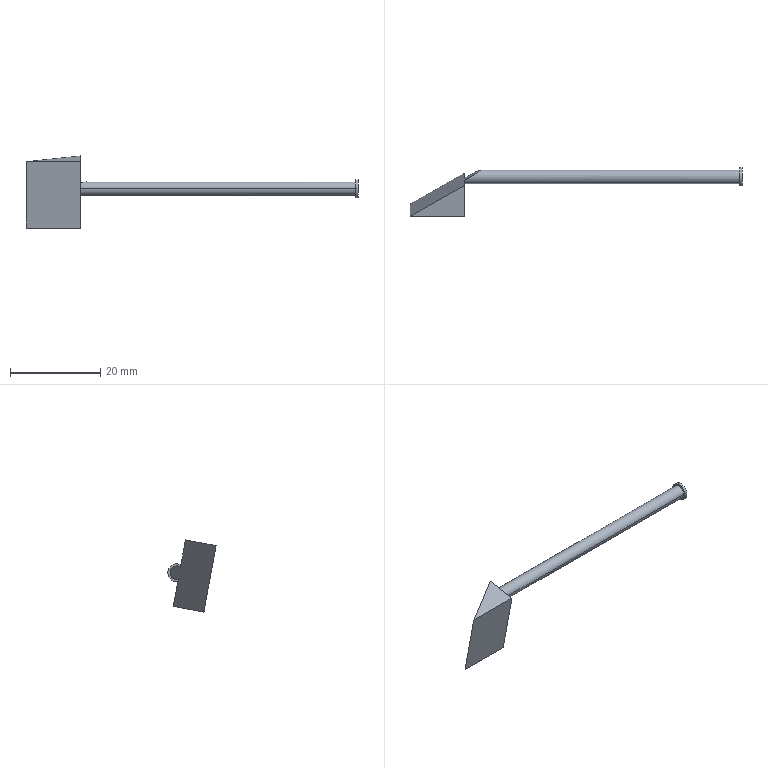Part | SolidWorks | features ICE 4, Cut 1, Helix 1, Revolution 1, Scale 1, SweepCut 1 | 1 solid | 11 faces | box 73.75 x 10.739 x 16.01 mm | volume 1055 mm3 | plane 7 | cylinder 4 | commonest cylinder face diameters 3 x2 4 x2
STEP:
#1=CARTESIAN_POINT('',(42.25,-1.5,0.));
#2=VERTEX_POINT('',#1);
#3=CARTESIAN_POINT('',(42.25,1.5,0.));
#4=VERTEX_POINT('',#3);
#5=CARTESIAN_POINT('',(42.25,0.,0.));
#6=DIRECTION('',(-1.,0.,0.));
#7=DIRECTION('',(0.,-1.,0.));
#8=AXIS2_PLACEMENT_3D('',#5,#6,#7);
#9=CIRCLE('',#8,1.5);
#10=EDGE_CURVE('',#2,#4,#9,.T.);
#11=ORIENTED_EDGE('',*,*,#10,.T.);
#12=CARTESIAN_POINT('',(-15.455,1.5,0.));
#13=VERTEX_POINT('',#12);
#14=CARTESIAN_POINT('',(-11.,1.5,0.));
#15=DIRECTION('',(-1.,0.,0.));
#16=VECTOR('',#15,1000.);
#17=LINE('',#14,#16);
#18=EDGE_CURVE('',#4,#13,#17,.T.);
#19=ORIENTED_EDGE('',*,*,#18,.T.);
#20=CARTESIAN_POINT('',(-19.,-0.8145,1.26));
#21=VERTEX_POINT('',#20);
#22=CARTESIAN_POINT('',(-15.455,1.5,0.));
#23=CARTESIAN_POINT('',(-15.031,1.5,1.347));
#24=CARTESIAN_POINT('',(-16.843,0.3168,1.991));
#25=CARTESIAN_POINT('',(-19.,-0.8145,1.26));
#26=(BOUNDED_CURVE()B_SPLINE_CURVE(3,(#22,#23,#24,#25),.UNSPECIFIED.,.F.,.F.)B_SPLINE_CURVE_WITH_KNOTS((4,4),(2.959,5.103),.UNSPECIFIED.)CURVE()GEOMETRIC_REPRESENTATION_ITEM()RATIONAL_B_SPLINE_CURVE((1.,0.652,0.652,1.))REPRESENTATION_ITEM(''));
#27=EDGE_CURVE('',#13,#21,#26,.T.);
#28=ORIENTED_EDGE('',*,*,#27,.T.);
#29=CARTESIAN_POINT('',(-19.,-1.5,0.));
#30=VERTEX_POINT('',#29);
#31=CARTESIAN_POINT('',(-19.,0.,0.));
#32=DIRECTION('',(-1.,0.,0.));
#33=DIRECTION('',(0.,0.,1.));
#34=AXIS2_PLACEMENT_3D('',#31,#32,#33);
#35=CIRCLE('',#34,1.5);
#36=EDGE_CURVE('',#30,#21,#35,.T.);
#37=ORIENTED_EDGE('',*,*,#36,.F.);
#38=CARTESIAN_POINT('',(-11.,-1.5,0.));
#39=DIRECTION('',(-1.,0.,0.));
#40=VECTOR('',#39,1000.);
#41=LINE('',#38,#40);
#42=EDGE_CURVE('',#2,#30,#41,.T.);
#43=ORIENTED_EDGE('',*,*,#42,.F.);
#44=EDGE_LOOP('',(#11,#19,#28,#37,#43));
#45=FACE_OUTER_BOUND('',#44,.T.);
#46=CARTESIAN_POINT('',(-11.,0.,0.));
#47=DIRECTION('',(-1.,0.,0.));
#48=DIRECTION('',(0.,-1.,0.));
#49=AXIS2_PLACEMENT_3D('',#46,#47,#48);
#50=CYLINDRICAL_SURFACE('',#49,1.5);
#51=ADVANCED_FACE('',(#45),#50,.T.);
#52=CARTESIAN_POINT('',(42.75,-2.,0.));
#53=VERTEX_POINT('',#52);
#54=CARTESIAN_POINT('',(42.75,2.,0.));
#55=VERTEX_POINT('',#54);
#56=CARTESIAN_POINT('',(42.75,0.,0.));
#57=DIRECTION('',(-1.,0.,0.));
#58=DIRECTION('',(0.,-1.,0.));
#59=AXIS2_PLACEMENT_3D('',#56,#57,#58);
#60=CIRCLE('',#59,2.);
#61=EDGE_CURVE('',#53,#55,#60,.T.);
#62=ORIENTED_EDGE('',*,*,#61,.T.);
#63=CARTESIAN_POINT('',(42.25,2.,0.));
#64=VERTEX_POINT('',#63);
#65=CARTESIAN_POINT('',(-11.,2.,0.));
#66=DIRECTION('',(-1.,0.,0.));
#67=VECTOR('',#66,1000.);
#68=LINE('',#65,#67);
#69=EDGE_CURVE('',#55,#64,#68,.T.);
#70=ORIENTED_EDGE('',*,*,#69,.T.);
#71=CARTESIAN_POINT('',(42.25,-2.,0.));
#72=VERTEX_POINT('',#71);
#73=CARTESIAN_POINT('',(42.25,0.,0.));
#74=DIRECTION('',(-1.,0.,0.));
#75=DIRECTION('',(0.,-1.,0.));
#76=AXIS2_PLACEMENT_3D('',#73,#74,#75);
#77=CIRCLE('',#76,2.);
#78=EDGE_CURVE('',#72,#64,#77,.T.);
#79=ORIENTED_EDGE('',*,*,#78,.F.);
#80=CARTESIAN_POINT('',(-11.,-2.,0.));
#81=DIRECTION('',(-1.,0.,0.));
#82=VECTOR('',#81,1000.);
#83=LINE('',#80,#82);
#84=EDGE_CURVE('',#53,#72,#83,.T.);
#85=ORIENTED_EDGE('',*,*,#84,.F.);
#86=EDGE_LOOP('',(#62,#70,#79,#85));
#87=FACE_OUTER_BOUND('',#86,.T.);
#88=CARTESIAN_POINT('',(-11.,0.,0.));
#89=DIRECTION('',(-1.,0.,0.));
#90=DIRECTION('',(0.,-1.,0.));
#91=AXIS2_PLACEMENT_3D('',#88,#89,#90);
#92=CYLINDRICAL_SURFACE('',#91,2.);
#93=ADVANCED_FACE('',(#87),#92,.T.);
#94=ORIENTED_EDGE('',*,*,#10,.F.);
#95=CARTESIAN_POINT('',(42.25,0.,0.));
#96=DIRECTION('',(-1.,0.,0.));
#97=DIRECTION('',(0.,-1.,0.));
#98=AXIS2_PLACEMENT_3D('',#95,#96,#97);
#99=CIRCLE('',#98,1.5);
#100=EDGE_CURVE('',#4,#2,#99,.T.);
#101=ORIENTED_EDGE('',*,*,#100,.F.);
#102=EDGE_LOOP('',(#94,#101));
#103=FACE_BOUND('',#102,.T.);
#104=ORIENTED_EDGE('',*,*,#78,.T.);
#105=CARTESIAN_POINT('',(42.25,0.,0.));
#106=DIRECTION('',(-1.,0.,0.));
#107=DIRECTION('',(0.,-1.,0.));
#108=AXIS2_PLACEMENT_3D('',#105,#106,#107);
#109=CIRCLE('',#108,2.);
#110=EDGE_CURVE('',#64,#72,#109,.T.);
#111=ORIENTED_EDGE('',*,*,#110,.T.);
#112=EDGE_LOOP('',(#104,#111));
#113=FACE_OUTER_BOUND('',#112,.T.);
#114=CARTESIAN_POINT('',(42.25,1.5,0.));
#115=DIRECTION('',(1.,0.,0.));
#116=DIRECTION('',(0.,1.,0.));
#117=AXIS2_PLACEMENT_3D('',#114,#115,#116);
#118=PLANE('',#117);
#119=ADVANCED_FACE('',(#103,#113),#118,.F.);
#120=ORIENTED_EDGE('',*,*,#69,.F.);
#121=CARTESIAN_POINT('',(42.75,0.,0.));
#122=DIRECTION('',(-1.,0.,0.));
#123=DIRECTION('',(0.,-1.,0.));
#124=AXIS2_PLACEMENT_3D('',#121,#122,#123);
#125=CIRCLE('',#124,2.);
#126=EDGE_CURVE('',#55,#53,#125,.T.);
#127=ORIENTED_EDGE('',*,*,#126,.T.);
#128=ORIENTED_EDGE('',*,*,#84,.T.);
#129=ORIENTED_EDGE('',*,*,#110,.F.);
#130=EDGE_LOOP('',(#120,#127,#128,#129));
#131=FACE_OUTER_BOUND('',#130,.T.);
#132=CARTESIAN_POINT('',(-11.,0.,0.));
#133=DIRECTION('',(-1.,0.,0.));
#134=DIRECTION('',(0.,-1.,0.));
#135=AXIS2_PLACEMENT_3D('',#132,#133,#134);
#136=CYLINDRICAL_SURFACE('',#135,2.);
#137=ADVANCED_FACE('',(#131),#136,.T.);
#138=ORIENTED_EDGE('',*,*,#61,.F.);
#139=ORIENTED_EDGE('',*,*,#126,.F.);
#140=EDGE_LOOP('',(#138,#139));
#141=FACE_OUTER_BOUND('',#140,.T.);
#142=CARTESIAN_POINT('',(42.75,2.,0.));
#143=DIRECTION('',(-1.,0.,0.));
#144=DIRECTION('',(0.,-1.,0.));
#145=AXIS2_PLACEMENT_3D('',#142,#143,#144);
#146=PLANE('',#145);
#147=ADVANCED_FACE('',(#141),#146,.F.);
#148=ORIENTED_EDGE('',*,*,#18,.F.);
#149=ORIENTED_EDGE('',*,*,#100,.T.);
#150=ORIENTED_EDGE('',*,*,#42,.T.);
#151=CARTESIAN_POINT('',(-19.,-0.31,-1.468));
#152=VERTEX_POINT('',#151);
#153=CARTESIAN_POINT('',(-19.,0.,0.));
#154=DIRECTION('',(-1.,0.,0.));
#155=DIRECTION('',(0.,0.,1.));
#156=AXIS2_PLACEMENT_3D('',#153,#154,#155);
#157=CIRCLE('',#156,1.5);
#158=EDGE_CURVE('',#152,#30,#157,.T.);
#159=ORIENTED_EDGE('',*,*,#158,.F.);
#160=CARTESIAN_POINT('',(-19.,-0.31,-1.468));
#161=CARTESIAN_POINT('',(-17.349,0.699,-1.681));
#162=CARTESIAN_POINT('',(-15.78,1.5,-1.031));
#163=CARTESIAN_POINT('',(-15.455,1.5,0.));
#164=(BOUNDED_CURVE()B_SPLINE_CURVE(3,(#160,#161,#162,#163),.UNSPECIFIED.,.F.,.F.)B_SPLINE_CURVE_WITH_KNOTS((4,4),(1.18,2.959),.UNSPECIFIED.)CURVE()GEOMETRIC_REPRESENTATION_ITEM()RATIONAL_B_SPLINE_CURVE((1.,0.7532,0.7532,1.))REPRESENTATION_ITEM(''));
#165=EDGE_CURVE('',#152,#13,#164,.T.);
#166=ORIENTED_EDGE('',*,*,#165,.T.);
#167=EDGE_LOOP('',(#148,#149,#150,#159,#166));
#168=FACE_OUTER_BOUND('',#167,.T.);
#169=CARTESIAN_POINT('',(-11.,0.,0.));
#170=DIRECTION('',(-1.,0.,0.));
#171=DIRECTION('',(0.,-1.,0.));
#172=AXIS2_PLACEMENT_3D('',#169,#170,#171);
#173=CYLINDRICAL_SURFACE('',#172,1.5);
#174=ADVANCED_FACE('',(#168),#173,.T.);
#175=CARTESIAN_POINT('',(-19.,-6.011,-8.739));
#176=VERTEX_POINT('',#175);
#177=CARTESIAN_POINT('',(-19.,-8.739,6.011));
#178=VERTEX_POINT('',#177);
#179=CARTESIAN_POINT('',(-19.,-8.739,6.011));
#180=DIRECTION('',(0.,-0.1819,0.9833));
#181=VECTOR('',#180,1000.);
#182=LINE('',#179,#181);
#183=EDGE_CURVE('',#176,#178,#182,.T.);
#184=ORIENTED_EDGE('',*,*,#183,.T.);
#185=CARTESIAN_POINT('',(-31.,-8.739,6.011));
#186=VERTEX_POINT('',#185);
#187=CARTESIAN_POINT('',(-31.,-8.739,6.011));
#188=DIRECTION('',(1.,0.,0.));
#189=VECTOR('',#188,1000.);
#190=LINE('',#187,#189);
#191=EDGE_CURVE('',#186,#178,#190,.T.);
#192=ORIENTED_EDGE('',*,*,#191,.F.);
#193=CARTESIAN_POINT('',(-31.,-6.011,-8.739));
#194=VERTEX_POINT('',#193);
#195=CARTESIAN_POINT('',(-31.,-8.739,6.011));
#196=DIRECTION('',(0.,-0.1819,0.9833));
#197=VECTOR('',#196,1000.);
#198=LINE('',#195,#197);
#199=EDGE_CURVE('',#194,#186,#198,.T.);
#200=ORIENTED_EDGE('',*,*,#199,.F.);
#201=CARTESIAN_POINT('',(-31.,-6.011,-8.739));
#202=DIRECTION('',(1.,0.,0.));
#203=VECTOR('',#202,1000.);
#204=LINE('',#201,#203);
#205=EDGE_CURVE('',#194,#176,#204,.T.);
#206=ORIENTED_EDGE('',*,*,#205,.T.);
#207=EDGE_LOOP('',(#184,#192,#200,#206));
#208=FACE_OUTER_BOUND('',#207,.T.);
#209=CARTESIAN_POINT('',(-31.,-8.739,6.011));
#210=DIRECTION('',(0.,0.9833,0.1819));
#211=DIRECTION('',(0.,-0.1819,0.9833));
#212=AXIS2_PLACEMENT_3D('',#209,#210,#211);
#213=PLANE('',#212);
#214=ADVANCED_FACE('',(#208),#213,.F.);
#215=CARTESIAN_POINT('',(-19.,-1.926,7.271));
#216=VERTEX_POINT('',#215);
#217=CARTESIAN_POINT('',(-19.,6.011,8.739));
#218=DIRECTION('',(0.,0.9833,0.1819));
#219=VECTOR('',#218,1000.);
#220=LINE('',#217,#219);
#221=EDGE_CURVE('',#178,#216,#220,.T.);
#222=ORIENTED_EDGE('',*,*,#221,.T.);
#223=CARTESIAN_POINT('',(-24.505,-5.052,6.693));
#224=DIRECTION('',(-0.866,-0.4917,-0.09094));
#225=VECTOR('',#224,1000.);
#226=LINE('',#223,#225);
#227=EDGE_CURVE('',#216,#186,#226,.T.);
#228=ORIENTED_EDGE('',*,*,#227,.T.);
#229=ORIENTED_EDGE('',*,*,#191,.T.);
#230=EDGE_LOOP('',(#222,#228,#229));
#231=FACE_OUTER_BOUND('',#230,.T.);
#232=CARTESIAN_POINT('',(-31.,6.011,8.739));
#233=DIRECTION('',(0.,0.1819,-0.9833));
#234=DIRECTION('',(0.,0.9833,0.1819));
#235=AXIS2_PLACEMENT_3D('',#232,#233,#234);
#236=PLANE('',#235);
#237=ADVANCED_FACE('',(#231),#236,.F.);
#238=ORIENTED_EDGE('',*,*,#205,.F.);
#239=CARTESIAN_POINT('',(-19.,0.8018,-7.479));
#240=VERTEX_POINT('',#239);
#241=CARTESIAN_POINT('',(-5.019,8.739,-6.011));
#242=DIRECTION('',(-0.866,-0.4917,-0.09094));
#243=VECTOR('',#242,1000.);
#244=LINE('',#241,#243);
#245=EDGE_CURVE('',#240,#194,#244,.T.);
#246=ORIENTED_EDGE('',*,*,#245,.F.);
#247=CARTESIAN_POINT('',(-19.,-6.011,-8.739));
#248=DIRECTION('',(0.,-0.9833,-0.1819));
#249=VECTOR('',#248,1000.);
#250=LINE('',#247,#249);
#251=EDGE_CURVE('',#240,#176,#250,.T.);
#252=ORIENTED_EDGE('',*,*,#251,.T.);
#253=EDGE_LOOP('',(#238,#246,#252));
#254=FACE_OUTER_BOUND('',#253,.T.);
#255=CARTESIAN_POINT('',(-31.,-6.011,-8.739));
#256=DIRECTION('',(0.,-0.1819,0.9833));
#257=DIRECTION('',(0.,-0.9833,-0.1819));
#258=AXIS2_PLACEMENT_3D('',#255,#256,#257);
#259=PLANE('',#258);
#260=ADVANCED_FACE('',(#254),#259,.F.);
#261=CARTESIAN_POINT('',(-19.,-0.5623,-0.104));
#262=DIRECTION('',(0.,0.1819,-0.9833));
#263=VECTOR('',#262,1000.);
#264=LINE('',#261,#263);
#265=EDGE_CURVE('',#216,#21,#264,.T.);
#266=ORIENTED_EDGE('',*,*,#265,.F.);
#267=ORIENTED_EDGE('',*,*,#221,.F.);
#268=ORIENTED_EDGE('',*,*,#183,.F.);
#269=ORIENTED_EDGE('',*,*,#251,.F.);
#270=CARTESIAN_POINT('',(-19.,-0.5623,-0.104));
#271=DIRECTION('',(0.,0.1819,-0.9833));
#272=VECTOR('',#271,1000.);
#273=LINE('',#270,#272);
#274=EDGE_CURVE('',#152,#240,#273,.T.);
#275=ORIENTED_EDGE('',*,*,#274,.F.);
#276=ORIENTED_EDGE('',*,*,#158,.T.);
#277=ORIENTED_EDGE('',*,*,#36,.T.);
#278=EDGE_LOOP('',(#266,#267,#268,#269,#275,#276,#277));
#279=FACE_OUTER_BOUND('',#278,.T.);
#280=CARTESIAN_POINT('',(-19.,0.,0.));
#281=DIRECTION('',(1.,0.,0.));
#282=DIRECTION('',(0.,0.,-1.));
#283=AXIS2_PLACEMENT_3D('',#280,#281,#282);
#284=PLANE('',#283);
#285=ADVANCED_FACE('',(#279),#284,.T.);
#286=ORIENTED_EDGE('',*,*,#265,.T.);
#287=ORIENTED_EDGE('',*,*,#27,.F.);
#288=ORIENTED_EDGE('',*,*,#165,.F.);
#289=ORIENTED_EDGE('',*,*,#274,.T.);
#290=ORIENTED_EDGE('',*,*,#245,.T.);
#291=ORIENTED_EDGE('',*,*,#199,.T.);
#292=ORIENTED_EDGE('',*,*,#227,.F.);
#293=EDGE_LOOP('',(#286,#287,#288,#289,#290,#291,#292));
#294=FACE_OUTER_BOUND('',#293,.T.);
#295=CARTESIAN_POINT('',(-5.019,-0.173,42.172));
#296=DIRECTION('',(0.5,-0.8516,-0.1575));
#297=DIRECTION('',(0.8623,0.5063,0.));
#298=AXIS2_PLACEMENT_3D('',#295,#296,#297);
#299=PLANE('',#298);
#300=ADVANCED_FACE('',(#294),#299,.F.);
#301=CLOSED_SHELL('',(#51,#93,#119,#137,#147,#174,#214,#237,#260,#285,#300));
#302=MANIFOLD_SOLID_BREP('',#301);
#303=CARTESIAN_POINT('',(0.,0.,0.));
#304=DIRECTION('',(0.,0.,1.));
#305=DIRECTION('',(1.,0.,0.));
#306=AXIS2_PLACEMENT_3D('',#303,#304,#305);
#307=(LENGTH_UNIT()NAMED_UNIT(*)SI_UNIT(.MILLI.,.METRE.));
#308=UNCERTAINTY_MEASURE_WITH_UNIT(LENGTH_MEASURE(0.00001),#307,'','');
#309=(NAMED_UNIT(*)PLANE_ANGLE_UNIT()SI_UNIT($,.RADIAN.));
#310=(NAMED_UNIT(*)SI_UNIT($,.STERADIAN.)SOLID_ANGLE_UNIT());
#311=(GEOMETRIC_REPRESENTATION_CONTEXT(3)GLOBAL_UNCERTAINTY_ASSIGNED_CONTEXT((#308))GLOBAL_UNIT_ASSIGNED_CONTEXT((#307,#309,#310))REPRESENTATION_CONTEXT('',''));
#312=ADVANCED_BREP_SHAPE_REPRESENTATION('',(#302,#306),#311);